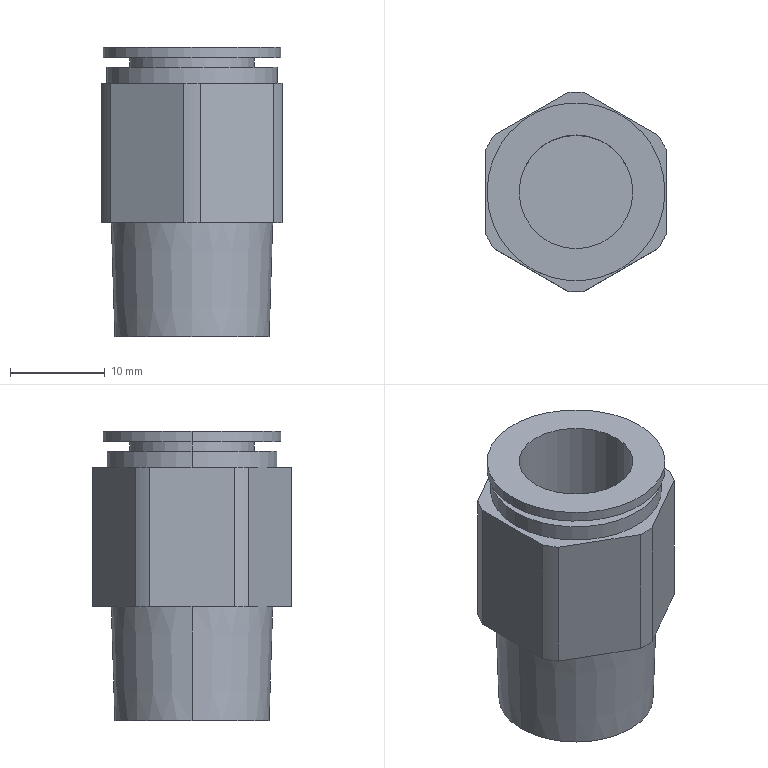Part | STEP file | GWS12-10 | 1 solid | 29 faces | box 19 x 21 x 30.5 mm | volume 5439 mm3 | cylinder 14 | plane 13 | cone 2 | commonest cylinder face diameters 21 x6 12 x2 13.1 x2 18 x2 18.75 x2